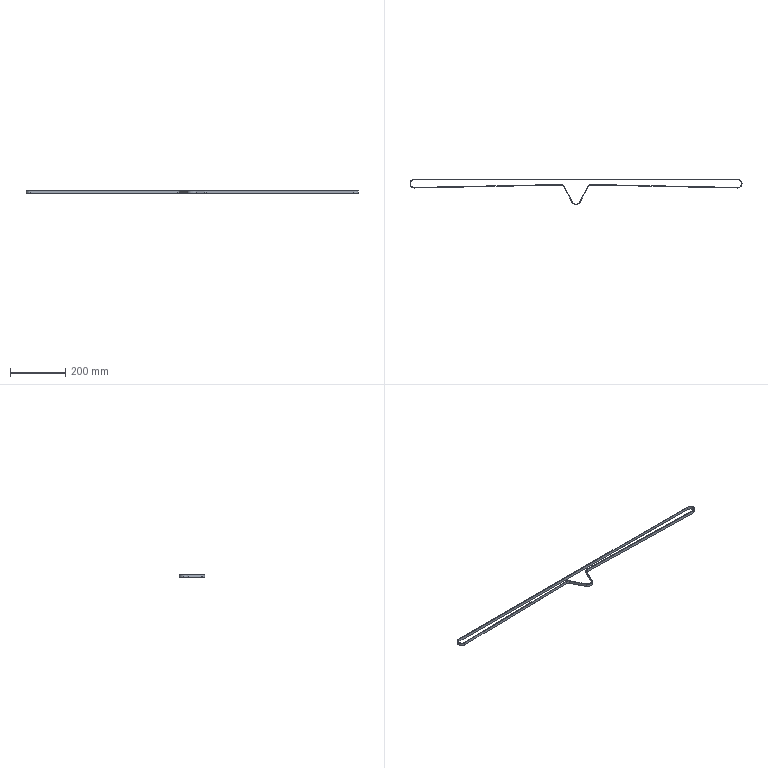Part | STEP file | 1 solid | 24 faces | box 1201 x 92.285 x 10 mm | volume 50245 mm3 | cylinder 12 | plane 12 | commonest cylinder face diameters 27.68 x3 31.68 x3 18 x2 22 x2 29.89 x1 33.89 x1